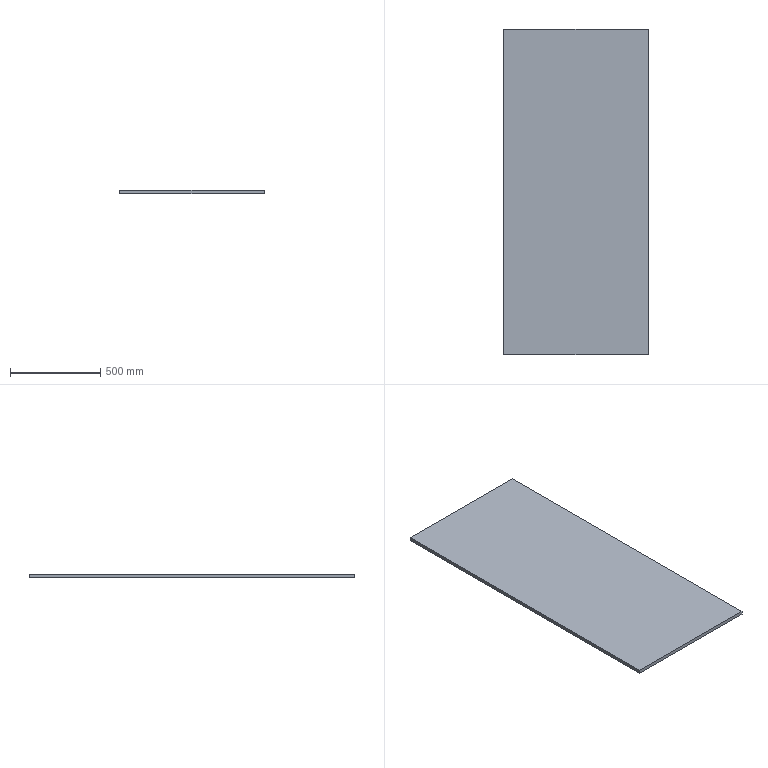Part | SolidWorks | features Extrusion 1 | 1 solid | 6 faces | box 800 x 1800 x 20 mm | volume 28800000 mm3 | plane 6
STEP:
#1=CARTESIAN_POINT('',(400.,-900.,0.));
#2=VERTEX_POINT('',#1);
#3=CARTESIAN_POINT('',(400.,900.,0.));
#4=VERTEX_POINT('',#3);
#5=CARTESIAN_POINT('',(400.,-900.,0.));
#6=DIRECTION('',(0.,1.,0.));
#7=VECTOR('',#6,1000.);
#8=LINE('',#5,#7);
#9=EDGE_CURVE('',#2,#4,#8,.T.);
#10=ORIENTED_EDGE('',*,*,#9,.T.);
#11=CARTESIAN_POINT('',(400.,900.,20.));
#12=VERTEX_POINT('',#11);
#13=CARTESIAN_POINT('',(400.,900.,20.));
#14=DIRECTION('',(0.,0.,-1.));
#15=VECTOR('',#14,1000.);
#16=LINE('',#13,#15);
#17=EDGE_CURVE('',#12,#4,#16,.T.);
#18=ORIENTED_EDGE('',*,*,#17,.F.);
#19=CARTESIAN_POINT('',(400.,-900.,20.));
#20=VERTEX_POINT('',#19);
#21=CARTESIAN_POINT('',(400.,-900.,20.));
#22=DIRECTION('',(0.,1.,0.));
#23=VECTOR('',#22,1000.);
#24=LINE('',#21,#23);
#25=EDGE_CURVE('',#20,#12,#24,.T.);
#26=ORIENTED_EDGE('',*,*,#25,.F.);
#27=CARTESIAN_POINT('',(400.,-900.,20.));
#28=DIRECTION('',(0.,0.,-1.));
#29=VECTOR('',#28,1000.);
#30=LINE('',#27,#29);
#31=EDGE_CURVE('',#20,#2,#30,.T.);
#32=ORIENTED_EDGE('',*,*,#31,.T.);
#33=EDGE_LOOP('',(#10,#18,#26,#32));
#34=FACE_OUTER_BOUND('',#33,.T.);
#35=CARTESIAN_POINT('',(400.,-900.,20.));
#36=DIRECTION('',(-1.,0.,0.));
#37=DIRECTION('',(0.,0.,1.));
#38=AXIS2_PLACEMENT_3D('',#35,#36,#37);
#39=PLANE('',#38);
#40=ADVANCED_FACE('',(#34),#39,.F.);
#41=CARTESIAN_POINT('',(-400.,900.,0.));
#42=VERTEX_POINT('',#41);
#43=CARTESIAN_POINT('',(-400.,900.,0.));
#44=DIRECTION('',(-1.,0.,0.));
#45=VECTOR('',#44,1000.);
#46=LINE('',#43,#45);
#47=EDGE_CURVE('',#4,#42,#46,.T.);
#48=ORIENTED_EDGE('',*,*,#47,.T.);
#49=CARTESIAN_POINT('',(-400.,900.,20.));
#50=VERTEX_POINT('',#49);
#51=CARTESIAN_POINT('',(-400.,900.,20.));
#52=DIRECTION('',(0.,0.,-1.));
#53=VECTOR('',#52,1000.);
#54=LINE('',#51,#53);
#55=EDGE_CURVE('',#50,#42,#54,.T.);
#56=ORIENTED_EDGE('',*,*,#55,.F.);
#57=CARTESIAN_POINT('',(-400.,900.,20.));
#58=DIRECTION('',(-1.,0.,0.));
#59=VECTOR('',#58,1000.);
#60=LINE('',#57,#59);
#61=EDGE_CURVE('',#12,#50,#60,.T.);
#62=ORIENTED_EDGE('',*,*,#61,.F.);
#63=ORIENTED_EDGE('',*,*,#17,.T.);
#64=EDGE_LOOP('',(#48,#56,#62,#63));
#65=FACE_OUTER_BOUND('',#64,.T.);
#66=CARTESIAN_POINT('',(-400.,900.,20.));
#67=DIRECTION('',(0.,-1.,0.));
#68=DIRECTION('',(0.,0.,-1.));
#69=AXIS2_PLACEMENT_3D('',#66,#67,#68);
#70=PLANE('',#69);
#71=ADVANCED_FACE('',(#65),#70,.F.);
#72=CARTESIAN_POINT('',(-400.,-900.,0.));
#73=VERTEX_POINT('',#72);
#74=CARTESIAN_POINT('',(-400.,-900.,0.));
#75=DIRECTION('',(0.,-1.,0.));
#76=VECTOR('',#75,1000.);
#77=LINE('',#74,#76);
#78=EDGE_CURVE('',#42,#73,#77,.T.);
#79=ORIENTED_EDGE('',*,*,#78,.T.);
#80=CARTESIAN_POINT('',(-400.,-900.,20.));
#81=VERTEX_POINT('',#80);
#82=CARTESIAN_POINT('',(-400.,-900.,20.));
#83=DIRECTION('',(0.,0.,-1.));
#84=VECTOR('',#83,1000.);
#85=LINE('',#82,#84);
#86=EDGE_CURVE('',#81,#73,#85,.T.);
#87=ORIENTED_EDGE('',*,*,#86,.F.);
#88=CARTESIAN_POINT('',(-400.,-900.,20.));
#89=DIRECTION('',(0.,-1.,0.));
#90=VECTOR('',#89,1000.);
#91=LINE('',#88,#90);
#92=EDGE_CURVE('',#50,#81,#91,.T.);
#93=ORIENTED_EDGE('',*,*,#92,.F.);
#94=ORIENTED_EDGE('',*,*,#55,.T.);
#95=EDGE_LOOP('',(#79,#87,#93,#94));
#96=FACE_OUTER_BOUND('',#95,.T.);
#97=CARTESIAN_POINT('',(-400.,-900.,20.));
#98=DIRECTION('',(1.,0.,0.));
#99=DIRECTION('',(0.,0.,-1.));
#100=AXIS2_PLACEMENT_3D('',#97,#98,#99);
#101=PLANE('',#100);
#102=ADVANCED_FACE('',(#96),#101,.F.);
#103=CARTESIAN_POINT('',(-400.,-900.,0.));
#104=DIRECTION('',(1.,0.,0.));
#105=VECTOR('',#104,1000.);
#106=LINE('',#103,#105);
#107=EDGE_CURVE('',#73,#2,#106,.T.);
#108=ORIENTED_EDGE('',*,*,#107,.T.);
#109=ORIENTED_EDGE('',*,*,#31,.F.);
#110=CARTESIAN_POINT('',(-400.,-900.,20.));
#111=DIRECTION('',(1.,0.,0.));
#112=VECTOR('',#111,1000.);
#113=LINE('',#110,#112);
#114=EDGE_CURVE('',#81,#20,#113,.T.);
#115=ORIENTED_EDGE('',*,*,#114,.F.);
#116=ORIENTED_EDGE('',*,*,#86,.T.);
#117=EDGE_LOOP('',(#108,#109,#115,#116));
#118=FACE_OUTER_BOUND('',#117,.T.);
#119=CARTESIAN_POINT('',(-400.,-900.,20.));
#120=DIRECTION('',(0.,1.,0.));
#121=DIRECTION('',(0.,0.,1.));
#122=AXIS2_PLACEMENT_3D('',#119,#120,#121);
#123=PLANE('',#122);
#124=ADVANCED_FACE('',(#118),#123,.F.);
#125=ORIENTED_EDGE('',*,*,#25,.T.);
#126=ORIENTED_EDGE('',*,*,#61,.T.);
#127=ORIENTED_EDGE('',*,*,#92,.T.);
#128=ORIENTED_EDGE('',*,*,#114,.T.);
#129=EDGE_LOOP('',(#125,#126,#127,#128));
#130=FACE_OUTER_BOUND('',#129,.T.);
#131=CARTESIAN_POINT('',(0.,0.,20.));
#132=DIRECTION('',(0.,0.,-1.));
#133=DIRECTION('',(-1.,0.,0.));
#134=AXIS2_PLACEMENT_3D('',#131,#132,#133);
#135=PLANE('',#134);
#136=ADVANCED_FACE('',(#130),#135,.F.);
#137=ORIENTED_EDGE('',*,*,#9,.F.);
#138=ORIENTED_EDGE('',*,*,#107,.F.);
#139=ORIENTED_EDGE('',*,*,#78,.F.);
#140=ORIENTED_EDGE('',*,*,#47,.F.);
#141=EDGE_LOOP('',(#137,#138,#139,#140));
#142=FACE_OUTER_BOUND('',#141,.T.);
#143=CARTESIAN_POINT('',(0.,0.,0.));
#144=DIRECTION('',(0.,0.,-1.));
#145=DIRECTION('',(-1.,0.,0.));
#146=AXIS2_PLACEMENT_3D('',#143,#144,#145);
#147=PLANE('',#146);
#148=ADVANCED_FACE('',(#142),#147,.T.);
#149=CLOSED_SHELL('',(#40,#71,#102,#124,#136,#148));
#150=MANIFOLD_SOLID_BREP('',#149);
#151=CARTESIAN_POINT('',(0.,0.,0.));
#152=DIRECTION('',(0.,0.,1.));
#153=DIRECTION('',(1.,0.,0.));
#154=AXIS2_PLACEMENT_3D('',#151,#152,#153);
#155=(LENGTH_UNIT()NAMED_UNIT(*)SI_UNIT(.MILLI.,.METRE.));
#156=UNCERTAINTY_MEASURE_WITH_UNIT(LENGTH_MEASURE(0.00001),#155,'','');
#157=(NAMED_UNIT(*)PLANE_ANGLE_UNIT()SI_UNIT($,.RADIAN.));
#158=(NAMED_UNIT(*)SI_UNIT($,.STERADIAN.)SOLID_ANGLE_UNIT());
#159=(GEOMETRIC_REPRESENTATION_CONTEXT(3)GLOBAL_UNCERTAINTY_ASSIGNED_CONTEXT((#156))GLOBAL_UNIT_ASSIGNED_CONTEXT((#155,#157,#158))REPRESENTATION_CONTEXT('',''));
#160=ADVANCED_BREP_SHAPE_REPRESENTATION('',(#150,#154),#159);